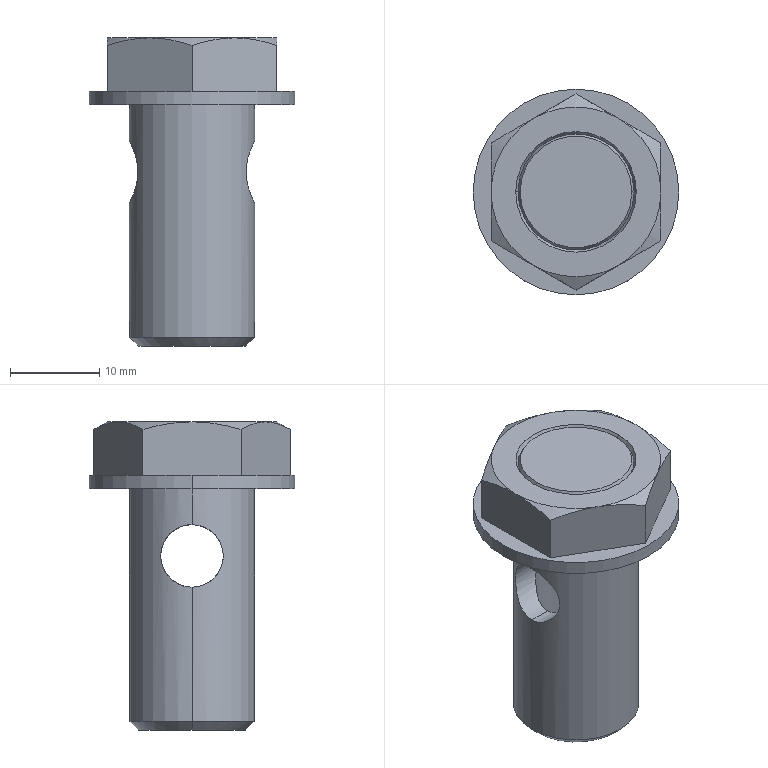Part | SolidWorks | features BaseBody 1 | 1 solid | 37 faces | box 23 x 23 x 34.5 mm | volume 4770 mm3 | cone 16 | plane 11 | cylinder 10 | commonest cylinder face diameters 7 x4 9 x2 14 x2 23 x2
STEP:
#1=CARTESIAN_POINT('',(49.25,110.5,76.5));
#2=VERTEX_POINT('',#1);
#3=CARTESIAN_POINT('',(61.75,110.5,76.5));
#4=VERTEX_POINT('',#3);
#5=CARTESIAN_POINT('',(55.5,110.5,76.5));
#6=DIRECTION('',(0.,0.,1.));
#7=DIRECTION('',(1.,0.,0.));
#8=AXIS2_PLACEMENT_3D('',#5,#6,#7);
#9=CIRCLE('',#8,6.25);
#10=EDGE_CURVE('',#2,#4,#9,.T.);
#11=ORIENTED_EDGE('',*,*,#10,.F.);
#12=CARTESIAN_POINT('',(49.,110.5,76.067));
#13=VERTEX_POINT('',#12);
#14=CARTESIAN_POINT('',(49.25,110.5,76.5));
#15=DIRECTION('',(-0.5,0.,-0.866));
#16=VECTOR('',#15,1000.);
#17=LINE('',#14,#16);
#18=EDGE_CURVE('',#2,#13,#17,.T.);
#19=ORIENTED_EDGE('',*,*,#18,.T.);
#20=CARTESIAN_POINT('',(62.,110.5,76.067));
#21=VERTEX_POINT('',#20);
#22=CARTESIAN_POINT('',(55.5,110.5,76.067));
#23=DIRECTION('',(0.,0.,1.));
#24=DIRECTION('',(1.,0.,0.));
#25=AXIS2_PLACEMENT_3D('',#22,#23,#24);
#26=CIRCLE('',#25,6.5);
#27=EDGE_CURVE('',#13,#21,#26,.T.);
#28=ORIENTED_EDGE('',*,*,#27,.T.);
#29=CARTESIAN_POINT('',(61.75,110.5,76.5));
#30=DIRECTION('',(0.5,0.,-0.866));
#31=VECTOR('',#30,1000.);
#32=LINE('',#29,#31);
#33=EDGE_CURVE('',#4,#21,#32,.T.);
#34=ORIENTED_EDGE('',*,*,#33,.F.);
#35=EDGE_LOOP('',(#11,#19,#28,#34));
#36=FACE_OUTER_BOUND('',#35,.T.);
#37=CARTESIAN_POINT('',(55.5,110.5,76.5));
#38=DIRECTION('',(0.,0.,-1.));
#39=DIRECTION('',(1.,0.,0.));
#40=AXIS2_PLACEMENT_3D('',#37,#38,#39);
#41=CONICAL_SURFACE('',#40,6.25,0.5236);
#42=ADVANCED_FACE('',(#36),#41,.T.);
#43=ORIENTED_EDGE('',*,*,#27,.F.);
#44=CARTESIAN_POINT('',(48.75,110.5,76.5));
#45=VERTEX_POINT('',#44);
#46=CARTESIAN_POINT('',(48.75,110.5,76.5));
#47=DIRECTION('',(-0.5,0.,0.866));
#48=VECTOR('',#47,1000.);
#49=LINE('',#46,#48);
#50=EDGE_CURVE('',#13,#45,#49,.T.);
#51=ORIENTED_EDGE('',*,*,#50,.T.);
#52=CARTESIAN_POINT('',(62.25,110.5,76.5));
#53=VERTEX_POINT('',#52);
#54=CARTESIAN_POINT('',(55.5,110.5,76.5));
#55=DIRECTION('',(0.,0.,1.));
#56=DIRECTION('',(1.,0.,0.));
#57=AXIS2_PLACEMENT_3D('',#54,#55,#56);
#58=CIRCLE('',#57,6.75);
#59=EDGE_CURVE('',#45,#53,#58,.T.);
#60=ORIENTED_EDGE('',*,*,#59,.T.);
#61=CARTESIAN_POINT('',(62.25,110.5,76.5));
#62=DIRECTION('',(0.5,0.,0.866));
#63=VECTOR('',#62,1000.);
#64=LINE('',#61,#63);
#65=EDGE_CURVE('',#21,#53,#64,.T.);
#66=ORIENTED_EDGE('',*,*,#65,.F.);
#67=EDGE_LOOP('',(#43,#51,#60,#66));
#68=FACE_OUTER_BOUND('',#67,.T.);
#69=CARTESIAN_POINT('',(55.5,110.5,76.5));
#70=DIRECTION('',(0.,0.,1.));
#71=DIRECTION('',(1.,0.,0.));
#72=AXIS2_PLACEMENT_3D('',#69,#70,#71);
#73=CONICAL_SURFACE('',#72,6.75,0.5236);
#74=ADVANCED_FACE('',(#68),#73,.F.);
#75=CARTESIAN_POINT('',(49.5,110.5,42.));
#76=VERTEX_POINT('',#75);
#77=CARTESIAN_POINT('',(61.5,110.5,42.));
#78=VERTEX_POINT('',#77);
#79=CARTESIAN_POINT('',(55.5,110.5,42.));
#80=DIRECTION('',(0.,0.,-1.));
#81=DIRECTION('',(-1.,0.,0.));
#82=AXIS2_PLACEMENT_3D('',#79,#80,#81);
#83=CIRCLE('',#82,6.);
#84=EDGE_CURVE('',#76,#78,#83,.T.);
#85=ORIENTED_EDGE('',*,*,#84,.F.);
#86=CARTESIAN_POINT('',(48.5,110.5,43.));
#87=VERTEX_POINT('',#86);
#88=CARTESIAN_POINT('',(49.5,110.5,42.));
#89=DIRECTION('',(-0.7071,0.,0.7071));
#90=VECTOR('',#89,1000.);
#91=LINE('',#88,#90);
#92=EDGE_CURVE('',#76,#87,#91,.T.);
#93=ORIENTED_EDGE('',*,*,#92,.T.);
#94=CARTESIAN_POINT('',(62.5,110.5,43.));
#95=VERTEX_POINT('',#94);
#96=CARTESIAN_POINT('',(55.5,110.5,43.));
#97=DIRECTION('',(0.,0.,1.));
#98=DIRECTION('',(-1.,0.,0.));
#99=AXIS2_PLACEMENT_3D('',#96,#97,#98);
#100=CIRCLE('',#99,7.);
#101=EDGE_CURVE('',#95,#87,#100,.T.);
#102=ORIENTED_EDGE('',*,*,#101,.F.);
#103=CARTESIAN_POINT('',(61.5,110.5,42.));
#104=DIRECTION('',(0.7071,0.,0.7071));
#105=VECTOR('',#104,1000.);
#106=LINE('',#103,#105);
#107=EDGE_CURVE('',#78,#95,#106,.T.);
#108=ORIENTED_EDGE('',*,*,#107,.F.);
#109=EDGE_LOOP('',(#85,#93,#102,#108));
#110=FACE_OUTER_BOUND('',#109,.T.);
#111=CARTESIAN_POINT('',(55.5,110.5,42.));
#112=DIRECTION('',(0.,0.,1.));
#113=DIRECTION('',(1.,0.,0.));
#114=AXIS2_PLACEMENT_3D('',#111,#112,#113);
#115=CONICAL_SURFACE('',#114,6.,0.7854);
#116=ADVANCED_FACE('',(#110),#115,.T.);
#117=CARTESIAN_POINT('',(60.,110.5,42.5));
#118=VERTEX_POINT('',#117);
#119=CARTESIAN_POINT('',(51.,110.5,42.5));
#120=VERTEX_POINT('',#119);
#121=CARTESIAN_POINT('',(55.5,110.5,42.5));
#122=DIRECTION('',(0.,0.,-1.));
#123=DIRECTION('',(-1.,0.,0.));
#124=AXIS2_PLACEMENT_3D('',#121,#122,#123);
#125=CIRCLE('',#124,4.5);
#126=EDGE_CURVE('',#118,#120,#125,.T.);
#127=ORIENTED_EDGE('',*,*,#126,.F.);
#128=CARTESIAN_POINT('',(60.5,110.5,42.));
#129=VERTEX_POINT('',#128);
#130=CARTESIAN_POINT('',(60.,110.5,42.5));
#131=DIRECTION('',(0.7071,0.,-0.7071));
#132=VECTOR('',#131,1000.);
#133=LINE('',#130,#132);
#134=EDGE_CURVE('',#118,#129,#133,.T.);
#135=ORIENTED_EDGE('',*,*,#134,.T.);
#136=CARTESIAN_POINT('',(50.5,110.5,42.));
#137=VERTEX_POINT('',#136);
#138=CARTESIAN_POINT('',(55.5,110.5,42.));
#139=DIRECTION('',(0.,0.,1.));
#140=DIRECTION('',(-1.,0.,0.));
#141=AXIS2_PLACEMENT_3D('',#138,#139,#140);
#142=CIRCLE('',#141,5.);
#143=EDGE_CURVE('',#137,#129,#142,.T.);
#144=ORIENTED_EDGE('',*,*,#143,.F.);
#145=CARTESIAN_POINT('',(51.,110.5,42.5));
#146=DIRECTION('',(-0.7071,0.,-0.7071));
#147=VECTOR('',#146,1000.);
#148=LINE('',#145,#147);
#149=EDGE_CURVE('',#120,#137,#148,.T.);
#150=ORIENTED_EDGE('',*,*,#149,.F.);
#151=EDGE_LOOP('',(#127,#135,#144,#150));
#152=FACE_OUTER_BOUND('',#151,.T.);
#153=CARTESIAN_POINT('',(55.5,110.5,42.5));
#154=DIRECTION('',(0.,0.,-1.));
#155=DIRECTION('',(-1.,0.,0.));
#156=AXIS2_PLACEMENT_3D('',#153,#154,#155);
#157=CONICAL_SURFACE('',#156,4.5,0.7854);
#158=ADVANCED_FACE('',(#152),#157,.F.);
#159=CARTESIAN_POINT('',(51.,110.5,58.));
#160=VERTEX_POINT('',#159);
#161=CARTESIAN_POINT('',(51.,110.5,65.));
#162=VERTEX_POINT('',#161);
#163=CARTESIAN_POINT('',(51.,110.5,58.));
#164=CARTESIAN_POINT('',(51.,110.379,58.));
#165=CARTESIAN_POINT('',(51.005,110.257,58.006));
#166=CARTESIAN_POINT('',(51.024,110.018,58.031));
#167=CARTESIAN_POINT('',(51.039,109.9,58.05));
#168=CARTESIAN_POINT('',(51.095,109.551,58.123));
#169=CARTESIAN_POINT('',(51.151,109.323,58.196));
#170=CARTESIAN_POINT('',(51.289,108.899,58.379));
#171=CARTESIAN_POINT('',(51.371,108.698,58.491));
#172=CARTESIAN_POINT('',(51.553,108.329,58.746));
#173=CARTESIAN_POINT('',(51.651,108.161,58.888));
#174=CARTESIAN_POINT('',(51.856,107.853,59.199));
#175=CARTESIAN_POINT('',(51.962,107.714,59.37));
#176=CARTESIAN_POINT('',(52.167,107.472,59.731));
#177=CARTESIAN_POINT('',(52.267,107.368,59.923));
#178=CARTESIAN_POINT('',(52.447,107.192,60.336));
#179=CARTESIAN_POINT('',(52.527,107.122,60.556));
#180=CARTESIAN_POINT('',(52.639,107.026,61.016));
#181=CARTESIAN_POINT('',(52.672,107.,61.259));
#182=CARTESIAN_POINT('',(52.672,107.,61.739));
#183=CARTESIAN_POINT('',(52.639,107.025,61.983));
#184=CARTESIAN_POINT('',(52.527,107.121,62.443));
#185=CARTESIAN_POINT('',(52.447,107.192,62.665));
#186=CARTESIAN_POINT('',(52.267,107.367,63.077));
#187=CARTESIAN_POINT('',(52.167,107.472,63.269));
#188=CARTESIAN_POINT('',(51.961,107.715,63.632));
#189=CARTESIAN_POINT('',(51.855,107.855,63.802));
#190=CARTESIAN_POINT('',(51.651,108.161,64.113));
#191=CARTESIAN_POINT('',(51.553,108.329,64.254));
#192=CARTESIAN_POINT('',(51.371,108.698,64.509));
#193=CARTESIAN_POINT('',(51.289,108.899,64.621));
#194=CARTESIAN_POINT('',(51.151,109.322,64.804));
#195=CARTESIAN_POINT('',(51.095,109.55,64.877));
#196=CARTESIAN_POINT('',(51.02,110.017,64.975));
#197=CARTESIAN_POINT('',(51.,110.256,65.));
#198=CARTESIAN_POINT('',(51.,110.5,65.));
#199=B_SPLINE_CURVE_WITH_KNOTS('',3,(#163,#164,#165,#166,#167,#168,#169,#170,#171,#172,#173,#174,#175,#176,#177,#178,#179,#180,#181,#182,#183,#184,#185,#186,#187,#188,#189,#190,#191,#192,#193,#194,#195,#196,#197,#198),.UNSPECIFIED.,.F.,.F.,(4,2,2,2,2,2,2,2,2,2,2,2,2,2,2,2,2,4),(0.01153,0.01188,0.01224,0.01296,0.01368,0.0144,0.01512,0.01584,0.01656,0.01727,0.01799,0.01871,0.01943,0.02015,0.02087,0.02159,0.02231,0.02302),.UNSPECIFIED.);
#200=EDGE_CURVE('',#160,#162,#199,.T.);
#201=ORIENTED_EDGE('',*,*,#200,.F.);
#202=CARTESIAN_POINT('',(48.5,110.5,58.));
#203=VERTEX_POINT('',#202);
#204=CARTESIAN_POINT('',(67.,110.5,58.));
#205=DIRECTION('',(-1.,0.,0.));
#206=VECTOR('',#205,1000.);
#207=LINE('',#204,#206);
#208=EDGE_CURVE('',#160,#203,#207,.T.);
#209=ORIENTED_EDGE('',*,*,#208,.T.);
#210=CARTESIAN_POINT('',(48.5,110.5,65.));
#211=VERTEX_POINT('',#210);
#212=CARTESIAN_POINT('',(48.5,110.5,65.));
#213=CARTESIAN_POINT('',(48.5,110.264,65.));
#214=CARTESIAN_POINT('',(48.512,110.034,64.976));
#215=CARTESIAN_POINT('',(48.557,109.581,64.885));
#216=CARTESIAN_POINT('',(48.591,109.356,64.816));
#217=CARTESIAN_POINT('',(48.674,108.933,64.638));
#218=CARTESIAN_POINT('',(48.724,108.734,64.53));
#219=CARTESIAN_POINT('',(48.834,108.356,64.276));
#220=CARTESIAN_POINT('',(48.893,108.181,64.131));
#221=CARTESIAN_POINT('',(49.013,107.864,63.813));
#222=CARTESIAN_POINT('',(49.074,107.72,63.638));
#223=CARTESIAN_POINT('',(49.19,107.467,63.261));
#224=CARTESIAN_POINT('',(49.243,107.36,63.063));
#225=CARTESIAN_POINT('',(49.334,107.184,62.643));
#226=CARTESIAN_POINT('',(49.373,107.115,62.419));
#227=CARTESIAN_POINT('',(49.424,107.023,61.966));
#228=CARTESIAN_POINT('',(49.438,107.,61.736));
#229=CARTESIAN_POINT('',(49.438,107.,61.27));
#230=CARTESIAN_POINT('',(49.424,107.023,61.034));
#231=CARTESIAN_POINT('',(49.373,107.115,60.581));
#232=CARTESIAN_POINT('',(49.335,107.183,60.359));
#233=CARTESIAN_POINT('',(49.243,107.361,59.936));
#234=CARTESIAN_POINT('',(49.189,107.468,59.736));
#235=CARTESIAN_POINT('',(49.074,107.721,59.36));
#236=CARTESIAN_POINT('',(49.012,107.866,59.184));
#237=CARTESIAN_POINT('',(48.892,108.184,58.867));
#238=CARTESIAN_POINT('',(48.833,108.357,58.723));
#239=CARTESIAN_POINT('',(48.723,108.736,58.468));
#240=CARTESIAN_POINT('',(48.673,108.937,58.36));
#241=CARTESIAN_POINT('',(48.591,109.357,58.184));
#242=CARTESIAN_POINT('',(48.557,109.58,58.115));
#243=CARTESIAN_POINT('',(48.512,110.037,58.023));
#244=CARTESIAN_POINT('',(48.5,110.268,58.));
#245=CARTESIAN_POINT('',(48.5,110.5,58.));
#246=B_SPLINE_CURVE_WITH_KNOTS('',3,(#212,#213,#214,#215,#216,#217,#218,#219,#220,#221,#222,#223,#224,#225,#226,#227,#228,#229,#230,#231,#232,#233,#234,#235,#236,#237,#238,#239,#240,#241,#242,#243,#244,#245),.UNSPECIFIED.,.F.,.F.,(4,2,2,2,2,2,2,2,2,2,2,2,2,2,2,2,4),(0.,0.0006958,0.001392,0.002088,0.002783,0.003479,0.004175,0.004871,0.005567,0.006263,0.006958,0.007654,0.00835,0.009046,0.009742,0.01044,0.01113),.UNSPECIFIED.);
#247=EDGE_CURVE('',#211,#203,#246,.T.);
#248=ORIENTED_EDGE('',*,*,#247,.F.);
#249=CARTESIAN_POINT('',(67.,110.5,65.));
#250=DIRECTION('',(-1.,0.,0.));
#251=VECTOR('',#250,1000.);
#252=LINE('',#249,#251);
#253=EDGE_CURVE('',#162,#211,#252,.T.);
#254=ORIENTED_EDGE('',*,*,#253,.F.);
#255=EDGE_LOOP('',(#201,#209,#248,#254));
#256=FACE_OUTER_BOUND('',#255,.T.);
#257=CARTESIAN_POINT('',(67.,110.5,61.5));
#258=DIRECTION('',(-1.,0.,0.));
#259=DIRECTION('',(0.,0.,1.));
#260=AXIS2_PLACEMENT_3D('',#257,#258,#259);
#261=CYLINDRICAL_SURFACE('',#260,3.5);
#262=ADVANCED_FACE('',(#256),#261,.F.);
#263=CARTESIAN_POINT('',(62.5,110.5,58.));
#264=VERTEX_POINT('',#263);
#265=CARTESIAN_POINT('',(62.5,110.5,65.));
#266=VERTEX_POINT('',#265);
#267=CARTESIAN_POINT('',(62.5,110.5,58.));
#268=CARTESIAN_POINT('',(62.5,110.264,58.));
#269=CARTESIAN_POINT('',(62.488,110.034,58.024));
#270=CARTESIAN_POINT('',(62.443,109.581,58.115));
#271=CARTESIAN_POINT('',(62.409,109.356,58.184));
#272=CARTESIAN_POINT('',(62.326,108.933,58.362));
#273=CARTESIAN_POINT('',(62.276,108.734,58.47));
#274=CARTESIAN_POINT('',(62.166,108.356,58.724));
#275=CARTESIAN_POINT('',(62.107,108.181,58.869));
#276=CARTESIAN_POINT('',(61.987,107.864,59.187));
#277=CARTESIAN_POINT('',(61.926,107.72,59.362));
#278=CARTESIAN_POINT('',(61.81,107.467,59.739));
#279=CARTESIAN_POINT('',(61.757,107.36,59.937));
#280=CARTESIAN_POINT('',(61.666,107.184,60.357));
#281=CARTESIAN_POINT('',(61.627,107.115,60.581));
#282=CARTESIAN_POINT('',(61.576,107.023,61.034));
#283=CARTESIAN_POINT('',(61.562,107.,61.264));
#284=CARTESIAN_POINT('',(61.562,107.,61.73));
#285=CARTESIAN_POINT('',(61.576,107.023,61.966));
#286=CARTESIAN_POINT('',(61.627,107.115,62.419));
#287=CARTESIAN_POINT('',(61.665,107.183,62.641));
#288=CARTESIAN_POINT('',(61.757,107.361,63.064));
#289=CARTESIAN_POINT('',(61.811,107.468,63.264));
#290=CARTESIAN_POINT('',(61.926,107.721,63.64));
#291=CARTESIAN_POINT('',(61.988,107.866,63.816));
#292=CARTESIAN_POINT('',(62.108,108.184,64.133));
#293=CARTESIAN_POINT('',(62.167,108.357,64.277));
#294=CARTESIAN_POINT('',(62.277,108.736,64.532));
#295=CARTESIAN_POINT('',(62.327,108.937,64.64));
#296=CARTESIAN_POINT('',(62.409,109.357,64.816));
#297=CARTESIAN_POINT('',(62.443,109.58,64.885));
#298=CARTESIAN_POINT('',(62.488,110.037,64.977));
#299=CARTESIAN_POINT('',(62.5,110.268,65.));
#300=CARTESIAN_POINT('',(62.5,110.5,65.));
#301=B_SPLINE_CURVE_WITH_KNOTS('',3,(#267,#268,#269,#270,#271,#272,#273,#274,#275,#276,#277,#278,#279,#280,#281,#282,#283,#284,#285,#286,#287,#288,#289,#290,#291,#292,#293,#294,#295,#296,#297,#298,#299,#300),.UNSPECIFIED.,.F.,.F.,(4,2,2,2,2,2,2,2,2,2,2,2,2,2,2,2,4),(0.,0.0006958,0.001392,0.002088,0.002783,0.003479,0.004175,0.004871,0.005567,0.006263,0.006958,0.007654,0.00835,0.009046,0.009742,0.01044,0.01113),.UNSPECIFIED.);
#302=EDGE_CURVE('',#264,#266,#301,.T.);
#303=ORIENTED_EDGE('',*,*,#302,.F.);
#304=CARTESIAN_POINT('',(60.,110.5,58.));
#305=VERTEX_POINT('',#304);
#306=CARTESIAN_POINT('',(67.,110.5,58.));
#307=DIRECTION('',(-1.,0.,0.));
#308=VECTOR('',#307,1000.);
#309=LINE('',#306,#308);
#310=EDGE_CURVE('',#264,#305,#309,.T.);
#311=ORIENTED_EDGE('',*,*,#310,.T.);
#312=CARTESIAN_POINT('',(60.,110.5,65.));
#313=VERTEX_POINT('',#312);
#314=CARTESIAN_POINT('',(60.,110.5,65.));
#315=CARTESIAN_POINT('',(60.,110.256,65.));
#316=CARTESIAN_POINT('',(59.98,110.018,64.975));
#317=CARTESIAN_POINT('',(59.905,109.552,64.878));
#318=CARTESIAN_POINT('',(59.849,109.324,64.804));
#319=CARTESIAN_POINT('',(59.712,108.9,64.621));
#320=CARTESIAN_POINT('',(59.629,108.699,64.51));
#321=CARTESIAN_POINT('',(59.447,108.33,64.255));
#322=CARTESIAN_POINT('',(59.349,108.161,64.113));
#323=CARTESIAN_POINT('',(59.144,107.854,63.801));
#324=CARTESIAN_POINT('',(59.038,107.715,63.631));
#325=CARTESIAN_POINT('',(58.833,107.472,63.269));
#326=CARTESIAN_POINT('',(58.733,107.368,63.078));
#327=CARTESIAN_POINT('',(58.553,107.192,62.664));
#328=CARTESIAN_POINT('',(58.473,107.121,62.444));
#329=CARTESIAN_POINT('',(58.361,107.026,61.984));
#330=CARTESIAN_POINT('',(58.328,107.,61.74));
#331=CARTESIAN_POINT('',(58.328,107.,61.26));
#332=CARTESIAN_POINT('',(58.361,107.026,61.016));
#333=CARTESIAN_POINT('',(58.474,107.122,60.555));
#334=CARTESIAN_POINT('',(58.554,107.192,60.334));
#335=CARTESIAN_POINT('',(58.734,107.368,59.922));
#336=CARTESIAN_POINT('',(58.833,107.473,59.73));
#337=CARTESIAN_POINT('',(59.04,107.717,59.367));
#338=CARTESIAN_POINT('',(59.146,107.856,59.196));
#339=CARTESIAN_POINT('',(59.35,108.162,58.886));
#340=CARTESIAN_POINT('',(59.448,108.33,58.744));
#341=CARTESIAN_POINT('',(59.63,108.701,58.489));
#342=CARTESIAN_POINT('',(59.712,108.901,58.378));
#343=CARTESIAN_POINT('',(59.85,109.325,58.195));
#344=CARTESIAN_POINT('',(59.906,109.553,58.122));
#345=CARTESIAN_POINT('',(59.981,110.02,58.025));
#346=CARTESIAN_POINT('',(60.,110.257,58.));
#347=CARTESIAN_POINT('',(60.,110.5,58.));
#348=B_SPLINE_CURVE_WITH_KNOTS('',3,(#314,#315,#316,#317,#318,#319,#320,#321,#322,#323,#324,#325,#326,#327,#328,#329,#330,#331,#332,#333,#334,#335,#336,#337,#338,#339,#340,#341,#342,#343,#344,#345,#346,#347),.UNSPECIFIED.,.F.,.F.,(4,2,2,2,2,2,2,2,2,2,2,2,2,2,2,2,4),(0.,0.0007203,0.001441,0.002161,0.002881,0.003602,0.004322,0.005042,0.005763,0.006483,0.007203,0.007923,0.008644,0.009364,0.01008,0.0108,0.01153),.UNSPECIFIED.);
#349=EDGE_CURVE('',#313,#305,#348,.T.);
#350=ORIENTED_EDGE('',*,*,#349,.F.);
#351=CARTESIAN_POINT('',(67.,110.5,65.));
#352=DIRECTION('',(-1.,0.,0.));
#353=VECTOR('',#352,1000.);
#354=LINE('',#351,#353);
#355=EDGE_CURVE('',#266,#313,#354,.T.);
#356=ORIENTED_EDGE('',*,*,#355,.F.);
#357=EDGE_LOOP('',(#303,#311,#350,#356));
#358=FACE_OUTER_BOUND('',#357,.T.);
#359=CARTESIAN_POINT('',(67.,110.5,61.5));
#360=DIRECTION('',(-1.,0.,0.));
#361=DIRECTION('',(0.,0.,1.));
#362=AXIS2_PLACEMENT_3D('',#359,#360,#361);
#363=CYLINDRICAL_SURFACE('',#362,3.5);
#364=ADVANCED_FACE('',(#358),#363,.F.);
#365=CARTESIAN_POINT('',(55.5,110.5,69.598));
#366=VERTEX_POINT('',#365);
#367=CARTESIAN_POINT('',(51.,110.5,67.));
#368=VERTEX_POINT('',#367);
#369=CARTESIAN_POINT('',(51.,110.5,67.));
#370=DIRECTION('',(-0.866,0.,-0.5));
#371=VECTOR('',#370,1000.);
#372=LINE('',#369,#371);
#373=EDGE_CURVE('',#366,#368,#372,.T.);
#374=ORIENTED_EDGE('',*,*,#373,.F.);
#375=CARTESIAN_POINT('',(60.,110.5,67.));
#376=VERTEX_POINT('',#375);
#377=CARTESIAN_POINT('',(60.,110.5,67.));
#378=DIRECTION('',(0.866,0.,-0.5));
#379=VECTOR('',#378,1000.);
#380=LINE('',#377,#379);
#381=EDGE_CURVE('',#366,#376,#380,.T.);
#382=ORIENTED_EDGE('',*,*,#381,.T.);
#383=CARTESIAN_POINT('',(55.5,110.5,67.));
#384=DIRECTION('',(0.,0.,-1.));
#385=DIRECTION('',(-1.,0.,0.));
#386=AXIS2_PLACEMENT_3D('',#383,#384,#385);
#387=CIRCLE('',#386,4.5);
#388=EDGE_CURVE('',#376,#368,#387,.T.);
#389=ORIENTED_EDGE('',*,*,#388,.T.);
#390=EDGE_LOOP('',(#374,#382,#389));
#391=FACE_OUTER_BOUND('',#390,.T.);
#392=CARTESIAN_POINT('',(55.5,110.5,67.));
#393=DIRECTION('',(0.,0.,-1.));
#394=DIRECTION('',(-1.,0.,0.));
#395=AXIS2_PLACEMENT_3D('',#392,#393,#394);
#396=CONICAL_SURFACE('',#395,4.5,1.047);
#397=ADVANCED_FACE('',(#391),#396,.F.);
#398=ORIENTED_EDGE('',*,*,#388,.F.);
#399=CARTESIAN_POINT('',(60.,110.5,67.));
#400=DIRECTION('',(0.,0.,-1.));
#401=VECTOR('',#400,1000.);
#402=LINE('',#399,#401);
#403=EDGE_CURVE('',#376,#313,#402,.T.);
#404=ORIENTED_EDGE('',*,*,#403,.T.);
#405=ORIENTED_EDGE('',*,*,#349,.T.);
#406=CARTESIAN_POINT('',(60.,110.5,67.));
#407=DIRECTION('',(0.,0.,-1.));
#408=VECTOR('',#407,1000.);
#409=LINE('',#406,#408);
#410=EDGE_CURVE('',#305,#118,#409,.T.);
#411=ORIENTED_EDGE('',*,*,#410,.T.);
#412=ORIENTED_EDGE('',*,*,#126,.T.);
#413=CARTESIAN_POINT('',(51.,110.5,67.));
#414=DIRECTION('',(0.,0.,-1.));
#415=VECTOR('',#414,1000.);
#416=LINE('',#413,#415);
#417=EDGE_CURVE('',#160,#120,#416,.T.);
#418=ORIENTED_EDGE('',*,*,#417,.F.);
#419=ORIENTED_EDGE('',*,*,#200,.T.);
#420=CARTESIAN_POINT('',(51.,110.5,67.));
#421=DIRECTION('',(0.,0.,-1.));
#422=VECTOR('',#421,1000.);
#423=LINE('',#420,#422);
#424=EDGE_CURVE('',#368,#162,#423,.T.);
#425=ORIENTED_EDGE('',*,*,#424,.F.);
#426=EDGE_LOOP('',(#398,#404,#405,#411,#412,#418,#419,#425));
#427=FACE_OUTER_BOUND('',#426,.T.);
#428=CARTESIAN_POINT('',(55.5,110.5,67.));
#429=DIRECTION('',(0.,0.,-1.));
#430=DIRECTION('',(-1.,0.,0.));
#431=AXIS2_PLACEMENT_3D('',#428,#429,#430);
#432=CYLINDRICAL_SURFACE('',#431,4.5);
#433=ADVANCED_FACE('',(#427),#432,.F.);
#434=ORIENTED_EDGE('',*,*,#101,.T.);
#435=CARTESIAN_POINT('',(48.5,110.5,42.));
#436=DIRECTION('',(0.,0.,1.));
#437=VECTOR('',#436,1000.);
#438=LINE('',#435,#437);
#439=EDGE_CURVE('',#87,#203,#438,.T.);
#440=ORIENTED_EDGE('',*,*,#439,.T.);
#441=CARTESIAN_POINT('',(48.5,110.5,58.));
#442=CARTESIAN_POINT('',(48.5,110.732,58.));
#443=CARTESIAN_POINT('',(48.512,110.968,58.024));
#444=CARTESIAN_POINT('',(48.557,111.422,58.116));
#445=CARTESIAN_POINT('',(48.59,111.642,58.183));
#446=CARTESIAN_POINT('',(48.674,112.068,58.362));
#447=CARTESIAN_POINT('',(48.724,112.268,58.471));
#448=CARTESIAN_POINT('',(48.833,112.643,58.724));
#449=CARTESIAN_POINT('',(48.893,112.82,58.869));
#450=CARTESIAN_POINT('',(49.014,113.137,59.188));
#451=CARTESIAN_POINT('',(49.074,113.279,59.361));
#452=CARTESIAN_POINT('',(49.189,113.531,59.736));
#453=CARTESIAN_POINT('',(49.243,113.641,59.939));
#454=CARTESIAN_POINT('',(49.334,113.816,60.357));
#455=CARTESIAN_POINT('',(49.372,113.884,60.575));
#456=CARTESIAN_POINT('',(49.424,113.976,61.032));
#457=CARTESIAN_POINT('',(49.438,114.,61.265));
#458=CARTESIAN_POINT('',(49.438,114.,61.728));
#459=CARTESIAN_POINT('',(49.424,113.977,61.962));
#460=CARTESIAN_POINT('',(49.373,113.885,62.418));
#461=CARTESIAN_POINT('',(49.336,113.818,62.637));
#462=CARTESIAN_POINT('',(49.198,113.553,63.272));
#463=CARTESIAN_POINT('',(49.074,113.296,63.653));
#464=CARTESIAN_POINT('',(48.893,112.818,64.132));
#465=CARTESIAN_POINT('',(48.834,112.644,64.275));
#466=CARTESIAN_POINT('',(48.725,112.27,64.528));
#467=CARTESIAN_POINT('',(48.674,112.066,64.638));
#468=CARTESIAN_POINT('',(48.591,111.645,64.815));
#469=CARTESIAN_POINT('',(48.558,111.426,64.883));
#470=CARTESIAN_POINT('',(48.512,110.971,64.976));
#471=CARTESIAN_POINT('',(48.5,110.735,65.));
#472=CARTESIAN_POINT('',(48.5,110.5,65.));
#473=B_SPLINE_CURVE_WITH_KNOTS('',3,(#441,#442,#443,#444,#445,#446,#447,#448,#449,#450,#451,#452,#453,#454,#455,#456,#457,#458,#459,#460,#461,#462,#463,#464,#465,#466,#467,#468,#469,#470,#471,#472),.UNSPECIFIED.,.F.,.F.,(4,2,2,2,2,2,2,2,2,2,2,2,2,2,2,4),(0.01113,0.01183,0.01252,0.01322,0.01391,0.01461,0.0153,0.016,0.01669,0.01739,0.01808,0.01947,0.02016,0.02086,0.02155,0.02225),.UNSPECIFIED.);
#474=EDGE_CURVE('',#203,#211,#473,.T.);
#475=ORIENTED_EDGE('',*,*,#474,.T.);
#476=CARTESIAN_POINT('',(48.5,110.5,69.));
#477=VERTEX_POINT('',#476);
#478=CARTESIAN_POINT('',(48.5,110.5,42.));
#479=DIRECTION('',(0.,0.,1.));
#480=VECTOR('',#479,1000.);
#481=LINE('',#478,#480);
#482=EDGE_CURVE('',#211,#477,#481,.T.);
#483=ORIENTED_EDGE('',*,*,#482,.T.);
#484=CARTESIAN_POINT('',(62.5,110.5,69.));
#485=VERTEX_POINT('',#484);
#486=CARTESIAN_POINT('',(55.5,110.5,69.));
#487=DIRECTION('',(0.,0.,-1.));
#488=DIRECTION('',(-1.,0.,0.));
#489=AXIS2_PLACEMENT_3D('',#486,#487,#488);
#490=CIRCLE('',#489,7.);
#491=EDGE_CURVE('',#477,#485,#490,.T.);
#492=ORIENTED_EDGE('',*,*,#491,.T.);
#493=CARTESIAN_POINT('',(62.5,110.5,42.));
#494=DIRECTION('',(0.,0.,1.));
#495=VECTOR('',#494,1000.);
#496=LINE('',#493,#495);
#497=EDGE_CURVE('',#266,#485,#496,.T.);
#498=ORIENTED_EDGE('',*,*,#497,.F.);
#499=CARTESIAN_POINT('',(62.5,110.5,65.));
#500=CARTESIAN_POINT('',(62.5,110.732,65.));
#501=CARTESIAN_POINT('',(62.488,110.968,64.976));
#502=CARTESIAN_POINT('',(62.443,111.422,64.884));
#503=CARTESIAN_POINT('',(62.41,111.642,64.817));
#504=CARTESIAN_POINT('',(62.326,112.068,64.638));
#505=CARTESIAN_POINT('',(62.276,112.268,64.529));
#506=CARTESIAN_POINT('',(62.167,112.643,64.276));
#507=CARTESIAN_POINT('',(62.107,112.82,64.131));
#508=CARTESIAN_POINT('',(61.986,113.137,63.812));
#509=CARTESIAN_POINT('',(61.926,113.279,63.639));
#510=CARTESIAN_POINT('',(61.811,113.531,63.264));
#511=CARTESIAN_POINT('',(61.757,113.641,63.061));
#512=CARTESIAN_POINT('',(61.666,113.816,62.643));
#513=CARTESIAN_POINT('',(61.628,113.884,62.425));
#514=CARTESIAN_POINT('',(61.576,113.976,61.968));
#515=CARTESIAN_POINT('',(61.562,114.,61.735));
#516=CARTESIAN_POINT('',(61.562,114.,61.272));
#517=CARTESIAN_POINT('',(61.576,113.977,61.038));
#518=CARTESIAN_POINT('',(61.627,113.885,60.582));
#519=CARTESIAN_POINT('',(61.664,113.818,60.363));
#520=CARTESIAN_POINT('',(61.802,113.553,59.728));
#521=CARTESIAN_POINT('',(61.926,113.296,59.347));
#522=CARTESIAN_POINT('',(62.107,112.818,58.868));
#523=CARTESIAN_POINT('',(62.166,112.644,58.725));
#524=CARTESIAN_POINT('',(62.275,112.27,58.472));
#525=CARTESIAN_POINT('',(62.326,112.066,58.362));
#526=CARTESIAN_POINT('',(62.409,111.645,58.185));
#527=CARTESIAN_POINT('',(62.442,111.426,58.117));
#528=CARTESIAN_POINT('',(62.488,110.971,58.024));
#529=CARTESIAN_POINT('',(62.5,110.735,58.));
#530=CARTESIAN_POINT('',(62.5,110.5,58.));
#531=B_SPLINE_CURVE_WITH_KNOTS('',3,(#499,#500,#501,#502,#503,#504,#505,#506,#507,#508,#509,#510,#511,#512,#513,#514,#515,#516,#517,#518,#519,#520,#521,#522,#523,#524,#525,#526,#527,#528,#529,#530),.UNSPECIFIED.,.F.,.F.,(4,2,2,2,2,2,2,2,2,2,2,2,2,2,2,4),(0.01113,0.01183,0.01252,0.01322,0.01391,0.01461,0.0153,0.016,0.01669,0.01739,0.01808,0.01947,0.02016,0.02086,0.02155,0.02225),.UNSPECIFIED.);
#532=EDGE_CURVE('',#266,#264,#531,.T.);
#533=ORIENTED_EDGE('',*,*,#532,.T.);
#534=CARTESIAN_POINT('',(62.5,110.5,42.));
#535=DIRECTION('',(0.,0.,1.));
#536=VECTOR('',#535,1000.);
#537=LINE('',#534,#536);
#538=EDGE_CURVE('',#95,#264,#537,.T.);
#539=ORIENTED_EDGE('',*,*,#538,.F.);
#540=EDGE_LOOP('',(#434,#440,#475,#483,#492,#498,#533,#539));
#541=FACE_OUTER_BOUND('',#540,.T.);
#542=CARTESIAN_POINT('',(55.5,110.5,42.));
#543=DIRECTION('',(0.,0.,1.));
#544=DIRECTION('',(1.,0.,0.));
#545=AXIS2_PLACEMENT_3D('',#542,#543,#544);
#546=CYLINDRICAL_SURFACE('',#545,7.);
#547=ADVANCED_FACE('',(#541),#546,.T.);
#548=CARTESIAN_POINT('',(44.,110.5,69.));
#549=VERTEX_POINT('',#548);
#550=CARTESIAN_POINT('',(67.,110.5,69.));
#551=VERTEX_POINT('',#550);
#552=CARTESIAN_POINT('',(55.5,110.5,69.));
#553=DIRECTION('',(0.,0.,-1.));
#554=DIRECTION('',(-1.,0.,0.));
#555=AXIS2_PLACEMENT_3D('',#552,#553,#554);
#556=CIRCLE('',#555,11.5);
#557=EDGE_CURVE('',#549,#551,#556,.T.);
#558=ORIENTED_EDGE('',*,*,#557,.F.);
#559=CARTESIAN_POINT('',(44.,110.5,70.5));
#560=VERTEX_POINT('',#559);
#561=CARTESIAN_POINT('',(44.,110.5,69.));
#562=DIRECTION('',(0.,0.,1.));
#563=VECTOR('',#562,1000.);
#564=LINE('',#561,#563);
#565=EDGE_CURVE('',#549,#560,#564,.T.);
#566=ORIENTED_EDGE('',*,*,#565,.T.);
#567=CARTESIAN_POINT('',(67.,110.5,70.5));
#568=VERTEX_POINT('',#567);
#569=CARTESIAN_POINT('',(55.5,110.5,70.5));
#570=DIRECTION('',(0.,0.,-1.));
#571=DIRECTION('',(-1.,0.,0.));
#572=AXIS2_PLACEMENT_3D('',#569,#570,#571);
#573=CIRCLE('',#572,11.5);
#574=EDGE_CURVE('',#560,#568,#573,.T.);
#575=ORIENTED_EDGE('',*,*,#574,.T.);
#576=CARTESIAN_POINT('',(67.,110.5,69.));
#577=DIRECTION('',(0.,0.,1.));
#578=VECTOR('',#577,1000.);
#579=LINE('',#576,#578);
#580=EDGE_CURVE('',#551,#568,#579,.T.);
#581=ORIENTED_EDGE('',*,*,#580,.F.);
#582=EDGE_LOOP('',(#558,#566,#575,#581));
#583=FACE_OUTER_BOUND('',#582,.T.);
#584=CARTESIAN_POINT('',(55.5,110.5,69.));
#585=DIRECTION('',(0.,0.,1.));
#586=DIRECTION('',(1.,0.,0.));
#587=AXIS2_PLACEMENT_3D('',#584,#585,#586);
#588=CYLINDRICAL_SURFACE('',#587,11.5);
#589=ADVANCED_FACE('',(#583),#588,.T.);
#590=CARTESIAN_POINT('',(55.5,121.47,75.651));
#591=VERTEX_POINT('',#590);
#592=CARTESIAN_POINT('',(50.75,118.727,76.5));
#593=VERTEX_POINT('',#592);
#594=CARTESIAN_POINT('',(55.5,121.47,75.651));
#595=CARTESIAN_POINT('',(54.723,121.021,75.911));
#596=CARTESIAN_POINT('',(53.94,120.569,76.124));
#597=CARTESIAN_POINT('',(52.358,119.656,76.419));
#598=CARTESIAN_POINT('',(51.559,119.194,76.5));
#599=CARTESIAN_POINT('',(50.75,118.727,76.5));
#600=B_SPLINE_CURVE_WITH_KNOTS('',3,(#594,#595,#596,#597,#598,#599),.UNSPECIFIED.,.F.,.F.,(4,2,4),(0.000000238,0.002775,0.00555),.UNSPECIFIED.);
#601=EDGE_CURVE('',#591,#593,#600,.T.);
#602=ORIENTED_EDGE('',*,*,#601,.F.);
#603=CARTESIAN_POINT('',(55.5,121.47,70.5));
#604=VERTEX_POINT('',#603);
#605=CARTESIAN_POINT('',(55.5,121.47,70.5));
#606=DIRECTION('',(0.,0.,1.));
#607=VECTOR('',#606,1000.);
#608=LINE('',#605,#607);
#609=EDGE_CURVE('',#604,#591,#608,.T.);
#610=ORIENTED_EDGE('',*,*,#609,.F.);
#611=CARTESIAN_POINT('',(46.,115.985,70.5));
#612=VERTEX_POINT('',#611);
#613=CARTESIAN_POINT('',(46.,115.985,70.5));
#614=DIRECTION('',(0.866,0.5,0.));
#615=VECTOR('',#614,1000.);
#616=LINE('',#613,#615);
#617=EDGE_CURVE('',#612,#604,#616,.T.);
#618=ORIENTED_EDGE('',*,*,#617,.F.);
#619=CARTESIAN_POINT('',(46.,115.985,75.651));
#620=VERTEX_POINT('',#619);
#621=CARTESIAN_POINT('',(46.,115.985,70.5));
#622=DIRECTION('',(0.,0.,1.));
#623=VECTOR('',#622,1000.);
#624=LINE('',#621,#623);
#625=EDGE_CURVE('',#612,#620,#624,.T.);
#626=ORIENTED_EDGE('',*,*,#625,.T.);
#627=CARTESIAN_POINT('',(50.75,118.727,76.5));
#628=CARTESIAN_POINT('',(50.347,118.495,76.5));
#629=CARTESIAN_POINT('',(49.942,118.261,76.48));
#630=CARTESIAN_POINT('',(49.141,117.798,76.402));
#631=CARTESIAN_POINT('',(48.743,117.569,76.345));
#632=CARTESIAN_POINT('',(47.557,116.884,76.123));
#633=CARTESIAN_POINT('',(46.775,116.432,75.91));
#634=CARTESIAN_POINT('',(46.,115.985,75.651));
#635=B_SPLINE_CURVE_WITH_KNOTS('',3,(#627,#628,#629,#630,#631,#632,#633,#634),.UNSPECIFIED.,.F.,.F.,(4,2,2,4),(0.00555,0.006932,0.008314,0.01108),.UNSPECIFIED.);
#636=EDGE_CURVE('',#593,#620,#635,.T.);
#637=ORIENTED_EDGE('',*,*,#636,.F.);
#638=EDGE_LOOP('',(#602,#610,#618,#626,#637));
#639=FACE_OUTER_BOUND('',#638,.T.);
#640=CARTESIAN_POINT('',(46.,115.985,70.5));
#641=DIRECTION('',(0.5,-0.866,0.));
#642=DIRECTION('',(-0.866,-0.5,0.));
#643=AXIS2_PLACEMENT_3D('',#640,#641,#642);
#644=PLANE('',#643);
#645=ADVANCED_FACE('',(#639),#644,.F.);
#646=CARTESIAN_POINT('',(65.,115.985,75.651));
#647=VERTEX_POINT('',#646);
#648=CARTESIAN_POINT('',(60.25,118.727,76.5));
#649=VERTEX_POINT('',#648);
#650=CARTESIAN_POINT('',(65.,115.985,75.651));
#651=CARTESIAN_POINT('',(64.223,116.433,75.911));
#652=CARTESIAN_POINT('',(63.44,116.885,76.124));
#653=CARTESIAN_POINT('',(61.858,117.799,76.419));
#654=CARTESIAN_POINT('',(61.059,118.26,76.5));
#655=CARTESIAN_POINT('',(60.25,118.727,76.5));
#656=B_SPLINE_CURVE_WITH_KNOTS('',3,(#650,#651,#652,#653,#654,#655),.UNSPECIFIED.,.F.,.F.,(4,2,4),(0.000000238,0.002775,0.00555),.UNSPECIFIED.);
#657=EDGE_CURVE('',#647,#649,#656,.T.);
#658=ORIENTED_EDGE('',*,*,#657,.F.);
#659=CARTESIAN_POINT('',(65.,115.985,70.5));
#660=VERTEX_POINT('',#659);
#661=CARTESIAN_POINT('',(65.,115.985,70.5));
#662=DIRECTION('',(0.,0.,1.));
#663=VECTOR('',#662,1000.);
#664=LINE('',#661,#663);
#665=EDGE_CURVE('',#660,#647,#664,.T.);
#666=ORIENTED_EDGE('',*,*,#665,.F.);
#667=CARTESIAN_POINT('',(55.5,121.47,70.5));
#668=DIRECTION('',(0.866,-0.5,0.));
#669=VECTOR('',#668,1000.);
#670=LINE('',#667,#669);
#671=EDGE_CURVE('',#604,#660,#670,.T.);
#672=ORIENTED_EDGE('',*,*,#671,.F.);
#673=ORIENTED_EDGE('',*,*,#609,.T.);
#674=CARTESIAN_POINT('',(60.25,118.727,76.5));
#675=CARTESIAN_POINT('',(59.847,118.96,76.5));
#676=CARTESIAN_POINT('',(59.442,119.194,76.48));
#677=CARTESIAN_POINT('',(58.641,119.656,76.402));
#678=CARTESIAN_POINT('',(58.243,119.886,76.345));
#679=CARTESIAN_POINT('',(57.057,120.571,76.123));
#680=CARTESIAN_POINT('',(56.275,121.022,75.91));
#681=CARTESIAN_POINT('',(55.5,121.47,75.651));
#682=B_SPLINE_CURVE_WITH_KNOTS('',3,(#674,#675,#676,#677,#678,#679,#680,#681),.UNSPECIFIED.,.F.,.F.,(4,2,2,4),(0.00555,0.006932,0.008314,0.01108),.UNSPECIFIED.);
#683=EDGE_CURVE('',#649,#591,#682,.T.);
#684=ORIENTED_EDGE('',*,*,#683,.F.);
#685=EDGE_LOOP('',(#658,#666,#672,#673,#684));
#686=FACE_OUTER_BOUND('',#685,.T.);
#687=CARTESIAN_POINT('',(55.5,121.47,70.5));
#688=DIRECTION('',(-0.5,-0.866,0.));
#689=DIRECTION('',(-0.866,0.5,0.));
#690=AXIS2_PLACEMENT_3D('',#687,#688,#689);
#691=PLANE('',#690);
#692=ADVANCED_FACE('',(#686),#691,.F.);
#693=CARTESIAN_POINT('',(65.,105.015,75.651));
#694=VERTEX_POINT('',#693);
#695=CARTESIAN_POINT('',(65.,110.5,76.5));
#696=VERTEX_POINT('',#695);
#697=CARTESIAN_POINT('',(65.,105.015,75.651));
#698=CARTESIAN_POINT('',(65.,105.908,75.909));
#699=CARTESIAN_POINT('',(65.,106.821,76.125));
#700=CARTESIAN_POINT('',(65.,108.651,76.42));
#701=CARTESIAN_POINT('',(65.,109.572,76.5));
#702=CARTESIAN_POINT('',(65.,110.5,76.5));
#703=B_SPLINE_CURVE_WITH_KNOTS('',3,(#697,#698,#699,#700,#701,#702),.UNSPECIFIED.,.F.,.F.,(4,2,4),(0.01012,0.0129,0.01567),.UNSPECIFIED.);
#704=EDGE_CURVE('',#694,#696,#703,.T.);
#705=ORIENTED_EDGE('',*,*,#704,.F.);
#706=CARTESIAN_POINT('',(65.,105.015,70.5));
#707=VERTEX_POINT('',#706);
#708=CARTESIAN_POINT('',(65.,105.015,70.5));
#709=DIRECTION('',(0.,0.,1.));
#710=VECTOR('',#709,1000.);
#711=LINE('',#708,#710);
#712=EDGE_CURVE('',#707,#694,#711,.T.);
#713=ORIENTED_EDGE('',*,*,#712,.F.);
#714=CARTESIAN_POINT('',(65.,115.985,70.5));
#715=DIRECTION('',(0.,-1.,0.));
#716=VECTOR('',#715,1000.);
#717=LINE('',#714,#716);
#718=EDGE_CURVE('',#660,#707,#717,.T.);
#719=ORIENTED_EDGE('',*,*,#718,.F.);
#720=ORIENTED_EDGE('',*,*,#665,.T.);
#721=CARTESIAN_POINT('',(65.,110.5,76.5));
#722=CARTESIAN_POINT('',(65.,110.964,76.5));
#723=CARTESIAN_POINT('',(65.,111.431,76.48));
#724=CARTESIAN_POINT('',(65.,112.365,76.402));
#725=CARTESIAN_POINT('',(65.,112.827,76.344));
#726=CARTESIAN_POINT('',(65.,114.199,76.121));
#727=CARTESIAN_POINT('',(65.,115.098,75.908));
#728=CARTESIAN_POINT('',(65.,115.985,75.651));
#729=B_SPLINE_CURVE_WITH_KNOTS('',3,(#721,#722,#723,#724,#725,#726,#727,#728),.UNSPECIFIED.,.F.,.F.,(4,2,2,4),(0.01567,0.01706,0.01845,0.02123),.UNSPECIFIED.);
#730=EDGE_CURVE('',#696,#647,#729,.T.);
#731=ORIENTED_EDGE('',*,*,#730,.F.);
#732=EDGE_LOOP('',(#705,#713,#719,#720,#731));
#733=FACE_OUTER_BOUND('',#732,.T.);
#734=CARTESIAN_POINT('',(65.,115.985,70.5));
#735=DIRECTION('',(-1.,0.,0.));
#736=DIRECTION('',(0.,0.,1.));
#737=AXIS2_PLACEMENT_3D('',#734,#735,#736);
#738=PLANE('',#737);
#739=ADVANCED_FACE('',(#733),#738,.F.);
#740=CARTESIAN_POINT('',(55.5,99.53,75.651));
#741=VERTEX_POINT('',#740);
#742=CARTESIAN_POINT('',(60.25,102.273,76.5));
#743=VERTEX_POINT('',#742);
#744=CARTESIAN_POINT('',(55.5,99.53,75.651));
#745=CARTESIAN_POINT('',(56.277,99.979,75.911));
#746=CARTESIAN_POINT('',(57.06,100.431,76.124));
#747=CARTESIAN_POINT('',(58.642,101.344,76.419));
#748=CARTESIAN_POINT('',(59.441,101.806,76.5));
#749=CARTESIAN_POINT('',(60.25,102.273,76.5));
#750=B_SPLINE_CURVE_WITH_KNOTS('',3,(#744,#745,#746,#747,#748,#749),.UNSPECIFIED.,.F.,.F.,(4,2,4),(0.000000238,0.002775,0.00555),.UNSPECIFIED.);
#751=EDGE_CURVE('',#741,#743,#750,.T.);
#752=ORIENTED_EDGE('',*,*,#751,.F.);
#753=CARTESIAN_POINT('',(55.5,99.53,70.5));
#754=VERTEX_POINT('',#753);
#755=CARTESIAN_POINT('',(55.5,99.53,70.5));
#756=DIRECTION('',(0.,0.,1.));
#757=VECTOR('',#756,1000.);
#758=LINE('',#755,#757);
#759=EDGE_CURVE('',#754,#741,#758,.T.);
#760=ORIENTED_EDGE('',*,*,#759,.F.);
#761=CARTESIAN_POINT('',(65.,105.015,70.5));
#762=DIRECTION('',(-0.866,-0.5,0.));
#763=VECTOR('',#762,1000.);
#764=LINE('',#761,#763);
#765=EDGE_CURVE('',#707,#754,#764,.T.);
#766=ORIENTED_EDGE('',*,*,#765,.F.);
#767=ORIENTED_EDGE('',*,*,#712,.T.);
#768=CARTESIAN_POINT('',(60.25,102.273,76.5));
#769=CARTESIAN_POINT('',(60.653,102.505,76.5));
#770=CARTESIAN_POINT('',(61.058,102.739,76.48));
#771=CARTESIAN_POINT('',(61.859,103.202,76.402));
#772=CARTESIAN_POINT('',(62.257,103.431,76.345));
#773=CARTESIAN_POINT('',(63.443,104.116,76.123));
#774=CARTESIAN_POINT('',(64.225,104.568,75.91));
#775=CARTESIAN_POINT('',(65.,105.015,75.651));
#776=B_SPLINE_CURVE_WITH_KNOTS('',3,(#768,#769,#770,#771,#772,#773,#774,#775),.UNSPECIFIED.,.F.,.F.,(4,2,2,4),(0.00555,0.006932,0.008314,0.01108),.UNSPECIFIED.);
#777=EDGE_CURVE('',#743,#694,#776,.T.);
#778=ORIENTED_EDGE('',*,*,#777,.F.);
#779=EDGE_LOOP('',(#752,#760,#766,#767,#778));
#780=FACE_OUTER_BOUND('',#779,.T.);
#781=CARTESIAN_POINT('',(65.,105.015,70.5));
#782=DIRECTION('',(-0.5,0.866,0.));
#783=DIRECTION('',(0.866,0.5,0.));
#784=AXIS2_PLACEMENT_3D('',#781,#782,#783);
#785=PLANE('',#784);
#786=ADVANCED_FACE('',(#780),#785,.F.);
#787=CARTESIAN_POINT('',(46.,105.015,75.651));
#788=VERTEX_POINT('',#787);
#789=CARTESIAN_POINT('',(50.75,102.273,76.5));
#790=VERTEX_POINT('',#789);
#791=CARTESIAN_POINT('',(46.,105.015,75.651));
#792=CARTESIAN_POINT('',(46.777,104.567,75.911));
#793=CARTESIAN_POINT('',(47.56,104.115,76.124));
#794=CARTESIAN_POINT('',(49.142,103.201,76.419));
#795=CARTESIAN_POINT('',(49.941,102.74,76.5));
#796=CARTESIAN_POINT('',(50.75,102.273,76.5));
#797=B_SPLINE_CURVE_WITH_KNOTS('',3,(#791,#792,#793,#794,#795,#796),.UNSPECIFIED.,.F.,.F.,(4,2,4),(0.000000238,0.002775,0.00555),.UNSPECIFIED.);
#798=EDGE_CURVE('',#788,#790,#797,.T.);
#799=ORIENTED_EDGE('',*,*,#798,.F.);
#800=CARTESIAN_POINT('',(46.,105.015,70.5));
#801=VERTEX_POINT('',#800);
#802=CARTESIAN_POINT('',(46.,105.015,70.5));
#803=DIRECTION('',(0.,0.,1.));
#804=VECTOR('',#803,1000.);
#805=LINE('',#802,#804);
#806=EDGE_CURVE('',#801,#788,#805,.T.);
#807=ORIENTED_EDGE('',*,*,#806,.F.);
#808=CARTESIAN_POINT('',(55.5,99.53,70.5));
#809=DIRECTION('',(-0.866,0.5,0.));
#810=VECTOR('',#809,1000.);
#811=LINE('',#808,#810);
#812=EDGE_CURVE('',#754,#801,#811,.T.);
#813=ORIENTED_EDGE('',*,*,#812,.F.);
#814=ORIENTED_EDGE('',*,*,#759,.T.);
#815=CARTESIAN_POINT('',(50.75,102.273,76.5));
#816=CARTESIAN_POINT('',(51.153,102.04,76.5));
#817=CARTESIAN_POINT('',(51.558,101.806,76.48));
#818=CARTESIAN_POINT('',(52.359,101.344,76.402));
#819=CARTESIAN_POINT('',(52.757,101.114,76.345));
#820=CARTESIAN_POINT('',(53.943,100.429,76.123));
#821=CARTESIAN_POINT('',(54.725,99.978,75.91));
#822=CARTESIAN_POINT('',(55.5,99.53,75.651));
#823=B_SPLINE_CURVE_WITH_KNOTS('',3,(#815,#816,#817,#818,#819,#820,#821,#822),.UNSPECIFIED.,.F.,.F.,(4,2,2,4),(0.00555,0.006932,0.008314,0.01108),.UNSPECIFIED.);
#824=EDGE_CURVE('',#790,#741,#823,.T.);
#825=ORIENTED_EDGE('',*,*,#824,.F.);
#826=EDGE_LOOP('',(#799,#807,#813,#814,#825));
#827=FACE_OUTER_BOUND('',#826,.T.);
#828=CARTESIAN_POINT('',(55.5,99.53,70.5));
#829=DIRECTION('',(0.5,0.866,0.));
#830=DIRECTION('',(0.866,-0.5,0.));
#831=AXIS2_PLACEMENT_3D('',#828,#829,#830);
#832=PLANE('',#831);
#833=ADVANCED_FACE('',(#827),#832,.F.);
#834=CARTESIAN_POINT('',(46.,110.5,76.5));
#835=VERTEX_POINT('',#834);
#836=CARTESIAN_POINT('',(46.,115.985,75.651));
#837=CARTESIAN_POINT('',(46.,115.098,75.908));
#838=CARTESIAN_POINT('',(46.,114.199,76.121));
#839=CARTESIAN_POINT('',(46.,112.827,76.344));
#840=CARTESIAN_POINT('',(46.,112.365,76.402));
#841=CARTESIAN_POINT('',(46.,111.431,76.48));
#842=CARTESIAN_POINT('',(46.,110.964,76.5));
#843=CARTESIAN_POINT('',(46.,110.5,76.5));
#844=B_SPLINE_CURVE_WITH_KNOTS('',3,(#836,#837,#838,#839,#840,#841,#842,#843),.UNSPECIFIED.,.F.,.F.,(4,2,2,4),(0.02845,0.03123,0.03262,0.03401),.UNSPECIFIED.);
#845=EDGE_CURVE('',#620,#835,#844,.T.);
#846=ORIENTED_EDGE('',*,*,#845,.F.);
#847=ORIENTED_EDGE('',*,*,#625,.F.);
#848=CARTESIAN_POINT('',(46.,105.015,70.5));
#849=DIRECTION('',(0.,1.,0.));
#850=VECTOR('',#849,1000.);
#851=LINE('',#848,#850);
#852=EDGE_CURVE('',#801,#612,#851,.T.);
#853=ORIENTED_EDGE('',*,*,#852,.F.);
#854=ORIENTED_EDGE('',*,*,#806,.T.);
#855=CARTESIAN_POINT('',(46.,110.5,76.5));
#856=CARTESIAN_POINT('',(46.,109.572,76.5));
#857=CARTESIAN_POINT('',(46.,108.651,76.42));
#858=CARTESIAN_POINT('',(46.,106.821,76.125));
#859=CARTESIAN_POINT('',(46.,105.908,75.909));
#860=CARTESIAN_POINT('',(46.,105.015,75.651));
#861=B_SPLINE_CURVE_WITH_KNOTS('',3,(#855,#856,#857,#858,#859,#860),.UNSPECIFIED.,.F.,.F.,(4,2,4),(0.03401,0.03678,0.03956),.UNSPECIFIED.);
#862=EDGE_CURVE('',#835,#788,#861,.T.);
#863=ORIENTED_EDGE('',*,*,#862,.F.);
#864=EDGE_LOOP('',(#846,#847,#853,#854,#863));
#865=FACE_OUTER_BOUND('',#864,.T.);
#866=CARTESIAN_POINT('',(46.,105.015,70.5));
#867=DIRECTION('',(1.,0.,0.));
#868=DIRECTION('',(0.,0.,-1.));
#869=AXIS2_PLACEMENT_3D('',#866,#867,#868);
#870=PLANE('',#869);
#871=ADVANCED_FACE('',(#865),#870,.F.);
#872=CARTESIAN_POINT('',(55.5,110.5,69.));
#873=DIRECTION('',(0.,0.,-1.));
#874=DIRECTION('',(-1.,0.,0.));
#875=AXIS2_PLACEMENT_3D('',#872,#873,#874);
#876=CIRCLE('',#875,11.5);
#877=EDGE_CURVE('',#551,#549,#876,.T.);
#878=ORIENTED_EDGE('',*,*,#877,.T.);
#879=ORIENTED_EDGE('',*,*,#557,.T.);
#880=EDGE_LOOP('',(#878,#879));
#881=FACE_OUTER_BOUND('',#880,.T.);
#882=CARTESIAN_POINT('',(55.5,110.5,69.));
#883=DIRECTION('',(0.,0.,-1.));
#884=DIRECTION('',(-1.,0.,0.));
#885=AXIS2_PLACEMENT_3D('',#882,#883,#884);
#886=CIRCLE('',#885,7.);
#887=EDGE_CURVE('',#485,#477,#886,.T.);
#888=ORIENTED_EDGE('',*,*,#887,.F.);
#889=ORIENTED_EDGE('',*,*,#491,.F.);
#890=EDGE_LOOP('',(#888,#889));
#891=FACE_BOUND('',#890,.T.);
#892=CARTESIAN_POINT('',(55.5,110.5,69.));
#893=DIRECTION('',(0.,0.,-1.));
#894=DIRECTION('',(-1.,0.,0.));
#895=AXIS2_PLACEMENT_3D('',#892,#893,#894);
#896=PLANE('',#895);
#897=ADVANCED_FACE('',(#881,#891),#896,.T.);
#898=CARTESIAN_POINT('',(55.5,110.5,70.5));
#899=DIRECTION('',(0.,0.,-1.));
#900=DIRECTION('',(-1.,0.,0.));
#901=AXIS2_PLACEMENT_3D('',#898,#899,#900);
#902=CIRCLE('',#901,11.5);
#903=EDGE_CURVE('',#568,#560,#902,.T.);
#904=ORIENTED_EDGE('',*,*,#903,.F.);
#905=ORIENTED_EDGE('',*,*,#574,.F.);
#906=EDGE_LOOP('',(#904,#905));
#907=FACE_OUTER_BOUND('',#906,.T.);
#908=ORIENTED_EDGE('',*,*,#852,.T.);
#909=ORIENTED_EDGE('',*,*,#617,.T.);
#910=ORIENTED_EDGE('',*,*,#671,.T.);
#911=ORIENTED_EDGE('',*,*,#718,.T.);
#912=ORIENTED_EDGE('',*,*,#765,.T.);
#913=ORIENTED_EDGE('',*,*,#812,.T.);
#914=EDGE_LOOP('',(#908,#909,#910,#911,#912,#913));
#915=FACE_BOUND('',#914,.T.);
#916=CARTESIAN_POINT('',(55.5,110.5,70.5));
#917=DIRECTION('',(0.,0.,-1.));
#918=DIRECTION('',(-1.,0.,0.));
#919=AXIS2_PLACEMENT_3D('',#916,#917,#918);
#920=PLANE('',#919);
#921=ADVANCED_FACE('',(#907,#915),#920,.F.);
#922=ORIENTED_EDGE('',*,*,#565,.F.);
#923=ORIENTED_EDGE('',*,*,#877,.F.);
#924=ORIENTED_EDGE('',*,*,#580,.T.);
#925=ORIENTED_EDGE('',*,*,#903,.T.);
#926=EDGE_LOOP('',(#922,#923,#924,#925));
#927=FACE_OUTER_BOUND('',#926,.T.);
#928=CARTESIAN_POINT('',(55.5,110.5,69.));
#929=DIRECTION('',(0.,0.,1.));
#930=DIRECTION('',(1.,0.,0.));
#931=AXIS2_PLACEMENT_3D('',#928,#929,#930);
#932=CYLINDRICAL_SURFACE('',#931,11.5);
#933=ADVANCED_FACE('',(#927),#932,.T.);
#934=ORIENTED_EDGE('',*,*,#439,.F.);
#935=CARTESIAN_POINT('',(55.5,110.5,43.));
#936=DIRECTION('',(0.,0.,1.));
#937=DIRECTION('',(-1.,0.,0.));
#938=AXIS2_PLACEMENT_3D('',#935,#936,#937);
#939=CIRCLE('',#938,7.);
#940=EDGE_CURVE('',#87,#95,#939,.T.);
#941=ORIENTED_EDGE('',*,*,#940,.T.);
#942=ORIENTED_EDGE('',*,*,#538,.T.);
#943=ORIENTED_EDGE('',*,*,#302,.T.);
#944=ORIENTED_EDGE('',*,*,#497,.T.);
#945=ORIENTED_EDGE('',*,*,#887,.T.);
#946=ORIENTED_EDGE('',*,*,#482,.F.);
#947=ORIENTED_EDGE('',*,*,#247,.T.);
#948=EDGE_LOOP('',(#934,#941,#942,#943,#944,#945,#946,#947));
#949=FACE_OUTER_BOUND('',#948,.T.);
#950=CARTESIAN_POINT('',(55.5,110.5,42.));
#951=DIRECTION('',(0.,0.,1.));
#952=DIRECTION('',(1.,0.,0.));
#953=AXIS2_PLACEMENT_3D('',#950,#951,#952);
#954=CYLINDRICAL_SURFACE('',#953,7.);
#955=ADVANCED_FACE('',(#949),#954,.T.);
#956=CARTESIAN_POINT('',(55.5,110.5,42.));
#957=DIRECTION('',(0.,0.,-1.));
#958=DIRECTION('',(-1.,0.,0.));
#959=AXIS2_PLACEMENT_3D('',#956,#957,#958);
#960=CIRCLE('',#959,6.);
#961=EDGE_CURVE('',#78,#76,#960,.T.);
#962=ORIENTED_EDGE('',*,*,#961,.T.);
#963=ORIENTED_EDGE('',*,*,#84,.T.);
#964=EDGE_LOOP('',(#962,#963));
#965=FACE_OUTER_BOUND('',#964,.T.);
#966=ORIENTED_EDGE('',*,*,#143,.T.);
#967=CARTESIAN_POINT('',(55.5,110.5,42.));
#968=DIRECTION('',(0.,0.,1.));
#969=DIRECTION('',(-1.,0.,0.));
#970=AXIS2_PLACEMENT_3D('',#967,#968,#969);
#971=CIRCLE('',#970,5.);
#972=EDGE_CURVE('',#129,#137,#971,.T.);
#973=ORIENTED_EDGE('',*,*,#972,.T.);
#974=EDGE_LOOP('',(#966,#973));
#975=FACE_BOUND('',#974,.T.);
#976=CARTESIAN_POINT('',(55.5,110.5,42.));
#977=DIRECTION('',(0.,0.,-1.));
#978=DIRECTION('',(-1.,0.,0.));
#979=AXIS2_PLACEMENT_3D('',#976,#977,#978);
#980=PLANE('',#979);
#981=ADVANCED_FACE('',(#965,#975),#980,.T.);
#982=ORIENTED_EDGE('',*,*,#403,.F.);
#983=CARTESIAN_POINT('',(55.5,110.5,67.));
#984=DIRECTION('',(0.,0.,-1.));
#985=DIRECTION('',(-1.,0.,0.));
#986=AXIS2_PLACEMENT_3D('',#983,#984,#985);
#987=CIRCLE('',#986,4.5);
#988=EDGE_CURVE('',#368,#376,#987,.T.);
#989=ORIENTED_EDGE('',*,*,#988,.F.);
#990=ORIENTED_EDGE('',*,*,#424,.T.);
#991=CARTESIAN_POINT('',(51.,110.5,65.));
#992=CARTESIAN_POINT('',(51.,110.744,65.));
#993=CARTESIAN_POINT('',(51.02,110.982,64.975));
#994=CARTESIAN_POINT('',(51.095,111.448,64.878));
#995=CARTESIAN_POINT('',(51.151,111.676,64.804));
#996=CARTESIAN_POINT('',(51.288,112.1,64.621));
#997=CARTESIAN_POINT('',(51.371,112.301,64.51));
#998=CARTESIAN_POINT('',(51.553,112.67,64.255));
#999=CARTESIAN_POINT('',(51.651,112.839,64.113));
#1000=CARTESIAN_POINT('',(51.856,113.146,63.801));
#1001=CARTESIAN_POINT('',(51.962,113.285,63.631));
#1002=CARTESIAN_POINT('',(52.167,113.528,63.269));
#1003=CARTESIAN_POINT('',(52.267,113.632,63.078));
#1004=CARTESIAN_POINT('',(52.447,113.808,62.664));
#1005=CARTESIAN_POINT('',(52.527,113.879,62.444));
#1006=CARTESIAN_POINT('',(52.639,113.974,61.984));
#1007=CARTESIAN_POINT('',(52.672,114.,61.74));
#1008=CARTESIAN_POINT('',(52.672,114.,61.26));
#1009=CARTESIAN_POINT('',(52.639,113.974,61.016));
#1010=CARTESIAN_POINT('',(52.526,113.878,60.555));
#1011=CARTESIAN_POINT('',(52.446,113.808,60.334));
#1012=CARTESIAN_POINT('',(52.266,113.632,59.922));
#1013=CARTESIAN_POINT('',(52.167,113.527,59.73));
#1014=CARTESIAN_POINT('',(51.96,113.283,59.367));
#1015=CARTESIAN_POINT('',(51.854,113.144,59.196));
#1016=CARTESIAN_POINT('',(51.65,112.838,58.886));
#1017=CARTESIAN_POINT('',(51.552,112.67,58.744));
#1018=CARTESIAN_POINT('',(51.37,112.299,58.489));
#1019=CARTESIAN_POINT('',(51.288,112.099,58.378));
#1020=CARTESIAN_POINT('',(51.15,111.675,58.195));
#1021=CARTESIAN_POINT('',(51.094,111.447,58.122));
#1022=CARTESIAN_POINT('',(51.019,110.98,58.025));
#1023=CARTESIAN_POINT('',(51.,110.743,58.));
#1024=CARTESIAN_POINT('',(51.,110.5,58.));
#1025=B_SPLINE_CURVE_WITH_KNOTS('',3,(#991,#992,#993,#994,#995,#996,#997,#998,#999,#1000,#1001,#1002,#1003,#1004,#1005,#1006,#1007,#1008,#1009,#1010,#1011,#1012,#1013,#1014,#1015,#1016,#1017,#1018,#1019,#1020,#1021,#1022,#1023,#1024),.UNSPECIFIED.,.F.,.F.,(4,2,2,2,2,2,2,2,2,2,2,2,2,2,2,2,4),(0.,0.0007203,0.001441,0.002161,0.002881,0.003602,0.004322,0.005042,0.005763,0.006483,0.007203,0.007923,0.008644,0.009364,0.01008,0.0108,0.01153),.UNSPECIFIED.);
#1026=EDGE_CURVE('',#162,#160,#1025,.T.);
#1027=ORIENTED_EDGE('',*,*,#1026,.T.);
#1028=ORIENTED_EDGE('',*,*,#417,.T.);
#1029=CARTESIAN_POINT('',(55.5,110.5,42.5));
#1030=DIRECTION('',(0.,0.,-1.));
#1031=DIRECTION('',(-1.,0.,0.));
#1032=AXIS2_PLACEMENT_3D('',#1029,#1030,#1031);
#1033=CIRCLE('',#1032,4.5);
#1034=EDGE_CURVE('',#120,#118,#1033,.T.);
#1035=ORIENTED_EDGE('',*,*,#1034,.T.);
#1036=ORIENTED_EDGE('',*,*,#410,.F.);
#1037=CARTESIAN_POINT('',(60.,110.5,58.));
#1038=CARTESIAN_POINT('',(60.,110.621,58.));
#1039=CARTESIAN_POINT('',(59.995,110.743,58.006));
#1040=CARTESIAN_POINT('',(59.976,110.982,58.031));
#1041=CARTESIAN_POINT('',(59.961,111.1,58.05));
#1042=CARTESIAN_POINT('',(59.905,111.449,58.123));
#1043=CARTESIAN_POINT('',(59.849,111.677,58.196));
#1044=CARTESIAN_POINT('',(59.711,112.101,58.379));
#1045=CARTESIAN_POINT('',(59.629,112.302,58.491));
#1046=CARTESIAN_POINT('',(59.447,112.671,58.746));
#1047=CARTESIAN_POINT('',(59.349,112.839,58.888));
#1048=CARTESIAN_POINT('',(59.144,113.147,59.199));
#1049=CARTESIAN_POINT('',(59.038,113.286,59.37));
#1050=CARTESIAN_POINT('',(58.833,113.528,59.731));
#1051=CARTESIAN_POINT('',(58.733,113.632,59.923));
#1052=CARTESIAN_POINT('',(58.553,113.808,60.336));
#1053=CARTESIAN_POINT('',(58.473,113.878,60.556));
#1054=CARTESIAN_POINT('',(58.361,113.974,61.016));
#1055=CARTESIAN_POINT('',(58.328,114.,61.259));
#1056=CARTESIAN_POINT('',(58.328,114.,61.739));
#1057=CARTESIAN_POINT('',(58.361,113.975,61.983));
#1058=CARTESIAN_POINT('',(58.473,113.879,62.443));
#1059=CARTESIAN_POINT('',(58.553,113.808,62.665));
#1060=CARTESIAN_POINT('',(58.733,113.633,63.077));
#1061=CARTESIAN_POINT('',(58.833,113.528,63.269));
#1062=CARTESIAN_POINT('',(59.039,113.285,63.632));
#1063=CARTESIAN_POINT('',(59.145,113.145,63.802));
#1064=CARTESIAN_POINT('',(59.349,112.839,64.113));
#1065=CARTESIAN_POINT('',(59.447,112.671,64.254));
#1066=CARTESIAN_POINT('',(59.629,112.302,64.509));
#1067=CARTESIAN_POINT('',(59.711,112.101,64.621));
#1068=CARTESIAN_POINT('',(59.849,111.678,64.804));
#1069=CARTESIAN_POINT('',(59.905,111.45,64.877));
#1070=CARTESIAN_POINT('',(59.98,110.983,64.975));
#1071=CARTESIAN_POINT('',(60.,110.744,65.));
#1072=CARTESIAN_POINT('',(60.,110.5,65.));
#1073=B_SPLINE_CURVE_WITH_KNOTS('',3,(#1037,#1038,#1039,#1040,#1041,#1042,#1043,#1044,#1045,#1046,#1047,#1048,#1049,#1050,#1051,#1052,#1053,#1054,#1055,#1056,#1057,#1058,#1059,#1060,#1061,#1062,#1063,#1064,#1065,#1066,#1067,#1068,#1069,#1070,#1071,#1072),.UNSPECIFIED.,.F.,.F.,(4,2,2,2,2,2,2,2,2,2,2,2,2,2,2,2,2,4),(0.01153,0.01188,0.01224,0.01296,0.01368,0.0144,0.01512,0.01584,0.01656,0.01727,0.01799,0.01871,0.01943,0.02015,0.02087,0.02159,0.02231,0.02302),.UNSPECIFIED.);
#1074=EDGE_CURVE('',#305,#313,#1073,.T.);
#1075=ORIENTED_EDGE('',*,*,#1074,.T.);
#1076=EDGE_LOOP('',(#982,#989,#990,#1027,#1028,#1035,#1036,#1075));
#1077=FACE_OUTER_BOUND('',#1076,.T.);
#1078=CARTESIAN_POINT('',(55.5,110.5,67.));
#1079=DIRECTION('',(0.,0.,-1.));
#1080=DIRECTION('',(-1.,0.,0.));
#1081=AXIS2_PLACEMENT_3D('',#1078,#1079,#1080);
#1082=CYLINDRICAL_SURFACE('',#1081,4.5);
#1083=ADVANCED_FACE('',(#1077),#1082,.F.);
#1084=ORIENTED_EDGE('',*,*,#381,.F.);
#1085=ORIENTED_EDGE('',*,*,#373,.T.);
#1086=ORIENTED_EDGE('',*,*,#988,.T.);
#1087=EDGE_LOOP('',(#1084,#1085,#1086));
#1088=FACE_OUTER_BOUND('',#1087,.T.);
#1089=CARTESIAN_POINT('',(55.5,110.5,67.));
#1090=DIRECTION('',(0.,0.,-1.));
#1091=DIRECTION('',(-1.,0.,0.));
#1092=AXIS2_PLACEMENT_3D('',#1089,#1090,#1091);
#1093=CONICAL_SURFACE('',#1092,4.5,1.047);
#1094=ADVANCED_FACE('',(#1088),#1093,.F.);
#1095=ORIENTED_EDGE('',*,*,#310,.F.);
#1096=ORIENTED_EDGE('',*,*,#532,.F.);
#1097=ORIENTED_EDGE('',*,*,#355,.T.);
#1098=ORIENTED_EDGE('',*,*,#1074,.F.);
#1099=EDGE_LOOP('',(#1095,#1096,#1097,#1098));
#1100=FACE_OUTER_BOUND('',#1099,.T.);
#1101=CARTESIAN_POINT('',(67.,110.5,61.5));
#1102=DIRECTION('',(-1.,0.,0.));
#1103=DIRECTION('',(0.,0.,1.));
#1104=AXIS2_PLACEMENT_3D('',#1101,#1102,#1103);
#1105=CYLINDRICAL_SURFACE('',#1104,3.5);
#1106=ADVANCED_FACE('',(#1100),#1105,.F.);
#1107=ORIENTED_EDGE('',*,*,#208,.F.);
#1108=ORIENTED_EDGE('',*,*,#1026,.F.);
#1109=ORIENTED_EDGE('',*,*,#253,.T.);
#1110=ORIENTED_EDGE('',*,*,#474,.F.);
#1111=EDGE_LOOP('',(#1107,#1108,#1109,#1110));
#1112=FACE_OUTER_BOUND('',#1111,.T.);
#1113=CARTESIAN_POINT('',(67.,110.5,61.5));
#1114=DIRECTION('',(-1.,0.,0.));
#1115=DIRECTION('',(0.,0.,1.));
#1116=AXIS2_PLACEMENT_3D('',#1113,#1114,#1115);
#1117=CYLINDRICAL_SURFACE('',#1116,3.5);
#1118=ADVANCED_FACE('',(#1112),#1117,.F.);
#1119=ORIENTED_EDGE('',*,*,#134,.F.);
#1120=ORIENTED_EDGE('',*,*,#1034,.F.);
#1121=ORIENTED_EDGE('',*,*,#149,.T.);
#1122=ORIENTED_EDGE('',*,*,#972,.F.);
#1123=EDGE_LOOP('',(#1119,#1120,#1121,#1122));
#1124=FACE_OUTER_BOUND('',#1123,.T.);
#1125=CARTESIAN_POINT('',(55.5,110.5,42.5));
#1126=DIRECTION('',(0.,0.,-1.));
#1127=DIRECTION('',(-1.,0.,0.));
#1128=AXIS2_PLACEMENT_3D('',#1125,#1126,#1127);
#1129=CONICAL_SURFACE('',#1128,4.5,0.7854);
#1130=ADVANCED_FACE('',(#1124),#1129,.F.);
#1131=ORIENTED_EDGE('',*,*,#798,.T.);
#1132=CARTESIAN_POINT('',(55.5,110.5,76.5));
#1133=DIRECTION('',(0.,0.,-1.));
#1134=DIRECTION('',(-1.,0.,0.));
#1135=AXIS2_PLACEMENT_3D('',#1132,#1133,#1134);
#1136=CIRCLE('',#1135,9.5);
#1137=EDGE_CURVE('',#790,#835,#1136,.T.);
#1138=ORIENTED_EDGE('',*,*,#1137,.T.);
#1139=ORIENTED_EDGE('',*,*,#862,.T.);
#1140=EDGE_LOOP('',(#1131,#1138,#1139));
#1141=FACE_OUTER_BOUND('',#1140,.T.);
#1142=CARTESIAN_POINT('',(55.5,110.5,76.5));
#1143=DIRECTION('',(0.,0.,-1.));
#1144=DIRECTION('',(1.,0.,0.));
#1145=AXIS2_PLACEMENT_3D('',#1142,#1143,#1144);
#1146=CONICAL_SURFACE('',#1145,9.5,1.047);
#1147=ADVANCED_FACE('',(#1141),#1146,.T.);
#1148=ORIENTED_EDGE('',*,*,#751,.T.);
#1149=CARTESIAN_POINT('',(55.5,110.5,76.5));
#1150=DIRECTION('',(0.,0.,-1.));
#1151=DIRECTION('',(-1.,0.,0.));
#1152=AXIS2_PLACEMENT_3D('',#1149,#1150,#1151);
#1153=CIRCLE('',#1152,9.5);
#1154=EDGE_CURVE('',#743,#790,#1153,.T.);
#1155=ORIENTED_EDGE('',*,*,#1154,.T.);
#1156=ORIENTED_EDGE('',*,*,#824,.T.);
#1157=EDGE_LOOP('',(#1148,#1155,#1156));
#1158=FACE_OUTER_BOUND('',#1157,.T.);
#1159=CARTESIAN_POINT('',(55.5,110.5,76.5));
#1160=DIRECTION('',(0.,0.,-1.));
#1161=DIRECTION('',(1.,0.,0.));
#1162=AXIS2_PLACEMENT_3D('',#1159,#1160,#1161);
#1163=CONICAL_SURFACE('',#1162,9.5,1.047);
#1164=ADVANCED_FACE('',(#1158),#1163,.T.);
#1165=ORIENTED_EDGE('',*,*,#704,.T.);
#1166=CARTESIAN_POINT('',(55.5,110.5,76.5));
#1167=DIRECTION('',(0.,0.,-1.));
#1168=DIRECTION('',(-1.,0.,0.));
#1169=AXIS2_PLACEMENT_3D('',#1166,#1167,#1168);
#1170=CIRCLE('',#1169,9.5);
#1171=EDGE_CURVE('',#696,#743,#1170,.T.);
#1172=ORIENTED_EDGE('',*,*,#1171,.T.);
#1173=ORIENTED_EDGE('',*,*,#777,.T.);
#1174=EDGE_LOOP('',(#1165,#1172,#1173));
#1175=FACE_OUTER_BOUND('',#1174,.T.);
#1176=CARTESIAN_POINT('',(55.5,110.5,76.5));
#1177=DIRECTION('',(0.,0.,-1.));
#1178=DIRECTION('',(1.,0.,0.));
#1179=AXIS2_PLACEMENT_3D('',#1176,#1177,#1178);
#1180=CONICAL_SURFACE('',#1179,9.5,1.047);
#1181=ADVANCED_FACE('',(#1175),#1180,.T.);
#1182=ORIENTED_EDGE('',*,*,#730,.T.);
#1183=ORIENTED_EDGE('',*,*,#657,.T.);
#1184=CARTESIAN_POINT('',(55.5,110.5,76.5));
#1185=DIRECTION('',(0.,0.,1.));
#1186=DIRECTION('',(1.,0.,0.));
#1187=AXIS2_PLACEMENT_3D('',#1184,#1185,#1186);
#1188=CIRCLE('',#1187,9.5);
#1189=EDGE_CURVE('',#696,#649,#1188,.T.);
#1190=ORIENTED_EDGE('',*,*,#1189,.F.);
#1191=EDGE_LOOP('',(#1182,#1183,#1190));
#1192=FACE_OUTER_BOUND('',#1191,.T.);
#1193=CARTESIAN_POINT('',(55.5,110.5,76.5));
#1194=DIRECTION('',(0.,0.,-1.));
#1195=DIRECTION('',(1.,0.,0.));
#1196=AXIS2_PLACEMENT_3D('',#1193,#1194,#1195);
#1197=CONICAL_SURFACE('',#1196,9.5,1.047);
#1198=ADVANCED_FACE('',(#1192),#1197,.T.);
#1199=ORIENTED_EDGE('',*,*,#683,.T.);
#1200=ORIENTED_EDGE('',*,*,#601,.T.);
#1201=CARTESIAN_POINT('',(55.5,110.5,76.5));
#1202=DIRECTION('',(0.,0.,-1.));
#1203=DIRECTION('',(-1.,0.,0.));
#1204=AXIS2_PLACEMENT_3D('',#1201,#1202,#1203);
#1205=CIRCLE('',#1204,9.5);
#1206=EDGE_CURVE('',#593,#649,#1205,.T.);
#1207=ORIENTED_EDGE('',*,*,#1206,.T.);
#1208=EDGE_LOOP('',(#1199,#1200,#1207));
#1209=FACE_OUTER_BOUND('',#1208,.T.);
#1210=CARTESIAN_POINT('',(55.5,110.5,76.5));
#1211=DIRECTION('',(0.,0.,-1.));
#1212=DIRECTION('',(1.,0.,0.));
#1213=AXIS2_PLACEMENT_3D('',#1210,#1211,#1212);
#1214=CONICAL_SURFACE('',#1213,9.5,1.047);
#1215=ADVANCED_FACE('',(#1209),#1214,.T.);
#1216=ORIENTED_EDGE('',*,*,#636,.T.);
#1217=ORIENTED_EDGE('',*,*,#845,.T.);
#1218=CARTESIAN_POINT('',(55.5,110.5,76.5));
#1219=DIRECTION('',(0.,0.,-1.));
#1220=DIRECTION('',(-1.,0.,0.));
#1221=AXIS2_PLACEMENT_3D('',#1218,#1219,#1220);
#1222=CIRCLE('',#1221,9.5);
#1223=EDGE_CURVE('',#835,#593,#1222,.T.);
#1224=ORIENTED_EDGE('',*,*,#1223,.T.);
#1225=EDGE_LOOP('',(#1216,#1217,#1224));
#1226=FACE_OUTER_BOUND('',#1225,.T.);
#1227=CARTESIAN_POINT('',(55.5,110.5,76.5));
#1228=DIRECTION('',(0.,0.,-1.));
#1229=DIRECTION('',(1.,0.,0.));
#1230=AXIS2_PLACEMENT_3D('',#1227,#1228,#1229);
#1231=CONICAL_SURFACE('',#1230,9.5,1.047);
#1232=ADVANCED_FACE('',(#1226),#1231,.T.);
#1233=CARTESIAN_POINT('',(55.5,110.5,76.5));
#1234=DIRECTION('',(0.,0.,1.));
#1235=DIRECTION('',(1.,0.,0.));
#1236=AXIS2_PLACEMENT_3D('',#1233,#1234,#1235);
#1237=CIRCLE('',#1236,6.75);
#1238=EDGE_CURVE('',#53,#45,#1237,.T.);
#1239=ORIENTED_EDGE('',*,*,#1238,.F.);
#1240=ORIENTED_EDGE('',*,*,#59,.F.);
#1241=EDGE_LOOP('',(#1239,#1240));
#1242=FACE_BOUND('',#1241,.T.);
#1243=ORIENTED_EDGE('',*,*,#1223,.F.);
#1244=ORIENTED_EDGE('',*,*,#1137,.F.);
#1245=ORIENTED_EDGE('',*,*,#1154,.F.);
#1246=ORIENTED_EDGE('',*,*,#1171,.F.);
#1247=ORIENTED_EDGE('',*,*,#1189,.T.);
#1248=ORIENTED_EDGE('',*,*,#1206,.F.);
#1249=EDGE_LOOP('',(#1243,#1244,#1245,#1246,#1247,#1248));
#1250=FACE_OUTER_BOUND('',#1249,.T.);
#1251=CARTESIAN_POINT('',(55.5,121.47,76.5));
#1252=DIRECTION('',(0.,0.,-1.));
#1253=DIRECTION('',(-1.,0.,0.));
#1254=AXIS2_PLACEMENT_3D('',#1251,#1252,#1253);
#1255=PLANE('',#1254);
#1256=ADVANCED_FACE('',(#1242,#1250),#1255,.F.);
#1257=ORIENTED_EDGE('',*,*,#92,.F.);
#1258=ORIENTED_EDGE('',*,*,#961,.F.);
#1259=ORIENTED_EDGE('',*,*,#107,.T.);
#1260=ORIENTED_EDGE('',*,*,#940,.F.);
#1261=EDGE_LOOP('',(#1257,#1258,#1259,#1260));
#1262=FACE_OUTER_BOUND('',#1261,.T.);
#1263=CARTESIAN_POINT('',(55.5,110.5,42.));
#1264=DIRECTION('',(0.,0.,1.));
#1265=DIRECTION('',(1.,0.,0.));
#1266=AXIS2_PLACEMENT_3D('',#1263,#1264,#1265);
#1267=CONICAL_SURFACE('',#1266,6.,0.7854);
#1268=ADVANCED_FACE('',(#1262),#1267,.T.);
#1269=ORIENTED_EDGE('',*,*,#50,.F.);
#1270=CARTESIAN_POINT('',(55.5,110.5,76.067));
#1271=DIRECTION('',(0.,0.,1.));
#1272=DIRECTION('',(1.,0.,0.));
#1273=AXIS2_PLACEMENT_3D('',#1270,#1271,#1272);
#1274=CIRCLE('',#1273,6.5);
#1275=EDGE_CURVE('',#21,#13,#1274,.T.);
#1276=ORIENTED_EDGE('',*,*,#1275,.F.);
#1277=ORIENTED_EDGE('',*,*,#65,.T.);
#1278=ORIENTED_EDGE('',*,*,#1238,.T.);
#1279=EDGE_LOOP('',(#1269,#1276,#1277,#1278));
#1280=FACE_OUTER_BOUND('',#1279,.T.);
#1281=CARTESIAN_POINT('',(55.5,110.5,76.5));
#1282=DIRECTION('',(0.,0.,1.));
#1283=DIRECTION('',(1.,0.,0.));
#1284=AXIS2_PLACEMENT_3D('',#1281,#1282,#1283);
#1285=CONICAL_SURFACE('',#1284,6.75,0.5236);
#1286=ADVANCED_FACE('',(#1280),#1285,.F.);
#1287=ORIENTED_EDGE('',*,*,#18,.F.);
#1288=CARTESIAN_POINT('',(55.5,110.5,76.5));
#1289=DIRECTION('',(0.,0.,1.));
#1290=DIRECTION('',(1.,0.,0.));
#1291=AXIS2_PLACEMENT_3D('',#1288,#1289,#1290);
#1292=CIRCLE('',#1291,6.25);
#1293=EDGE_CURVE('',#4,#2,#1292,.T.);
#1294=ORIENTED_EDGE('',*,*,#1293,.F.);
#1295=ORIENTED_EDGE('',*,*,#33,.T.);
#1296=ORIENTED_EDGE('',*,*,#1275,.T.);
#1297=EDGE_LOOP('',(#1287,#1294,#1295,#1296));
#1298=FACE_OUTER_BOUND('',#1297,.T.);
#1299=CARTESIAN_POINT('',(55.5,110.5,76.5));
#1300=DIRECTION('',(0.,0.,-1.));
#1301=DIRECTION('',(1.,0.,0.));
#1302=AXIS2_PLACEMENT_3D('',#1299,#1300,#1301);
#1303=CONICAL_SURFACE('',#1302,6.25,0.5236);
#1304=ADVANCED_FACE('',(#1298),#1303,.T.);
#1305=ORIENTED_EDGE('',*,*,#1293,.T.);
#1306=ORIENTED_EDGE('',*,*,#10,.T.);
#1307=EDGE_LOOP('',(#1305,#1306));
#1308=FACE_OUTER_BOUND('',#1307,.T.);
#1309=CARTESIAN_POINT('',(55.5,121.47,76.5));
#1310=DIRECTION('',(0.,0.,-1.));
#1311=DIRECTION('',(-1.,0.,0.));
#1312=AXIS2_PLACEMENT_3D('',#1309,#1310,#1311);
#1313=PLANE('',#1312);
#1314=ADVANCED_FACE('',(#1308),#1313,.F.);
#1315=CLOSED_SHELL('',(#42,#74,#116,#158,#262,#364,#397,#433,#547,#589,#645,#692,#739,#786,#833,#871,#897,#921,#933,#955,#981,#1083,#1094,#1106,#1118,#1130,#1147,#1164,#1181,#1198,#1215,#1232,#1256,#1268,#1286,#1304,#1314));
#1316=MANIFOLD_SOLID_BREP('',#1315);
#1317=CARTESIAN_POINT('',(0.,0.,0.));
#1318=DIRECTION('',(0.,0.,1.));
#1319=DIRECTION('',(1.,0.,0.));
#1320=AXIS2_PLACEMENT_3D('',#1317,#1318,#1319);
#1321=(LENGTH_UNIT()NAMED_UNIT(*)SI_UNIT(.MILLI.,.METRE.));
#1322=UNCERTAINTY_MEASURE_WITH_UNIT(LENGTH_MEASURE(0.00001),#1321,'','');
#1323=(NAMED_UNIT(*)PLANE_ANGLE_UNIT()SI_UNIT($,.RADIAN.));
#1324=(NAMED_UNIT(*)SI_UNIT($,.STERADIAN.)SOLID_ANGLE_UNIT());
#1325=(GEOMETRIC_REPRESENTATION_CONTEXT(3)GLOBAL_UNCERTAINTY_ASSIGNED_CONTEXT((#1322))GLOBAL_UNIT_ASSIGNED_CONTEXT((#1321,#1323,#1324))REPRESENTATION_CONTEXT('',''));
#1326=ADVANCED_BREP_SHAPE_REPRESENTATION('',(#1316,#1320),#1325);